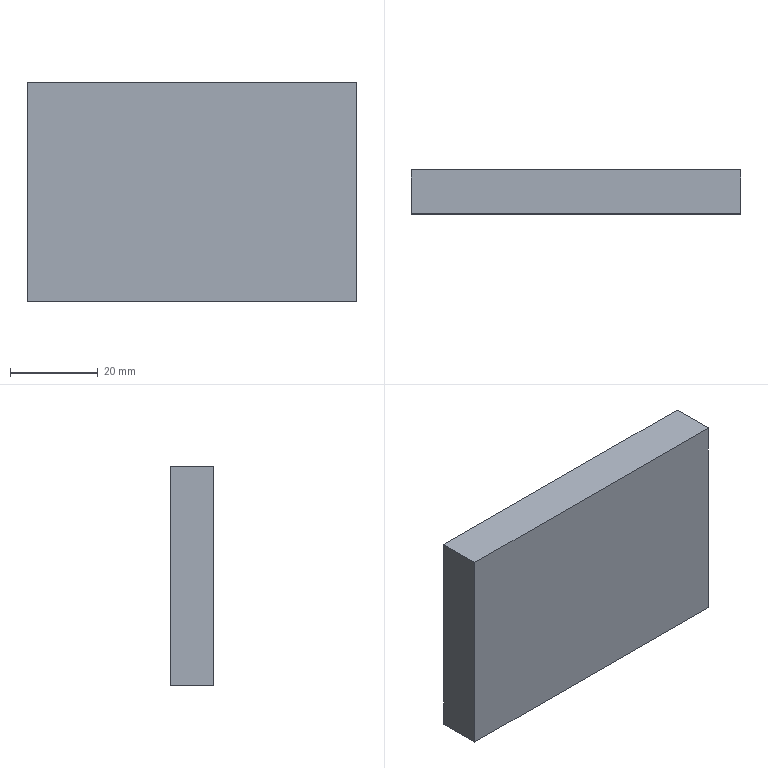Part | SolidWorks | features Extrusion 1 | 1 solid | 6 faces | box 75 x 10 x 50 mm | volume 37500 mm3 | plane 6
STEP:
#1=CARTESIAN_POINT('',(37.5,0.,25.));
#2=VERTEX_POINT('',#1);
#3=CARTESIAN_POINT('',(37.5,0.,-25.));
#4=VERTEX_POINT('',#3);
#5=CARTESIAN_POINT('',(37.5,0.,25.));
#6=DIRECTION('',(0.,0.,-1.));
#7=VECTOR('',#6,1000.);
#8=LINE('',#5,#7);
#9=EDGE_CURVE('',#2,#4,#8,.T.);
#10=ORIENTED_EDGE('',*,*,#9,.T.);
#11=CARTESIAN_POINT('',(37.5,10.,-25.));
#12=VERTEX_POINT('',#11);
#13=CARTESIAN_POINT('',(37.5,10.,-25.));
#14=DIRECTION('',(0.,-1.,0.));
#15=VECTOR('',#14,1000.);
#16=LINE('',#13,#15);
#17=EDGE_CURVE('',#12,#4,#16,.T.);
#18=ORIENTED_EDGE('',*,*,#17,.F.);
#19=CARTESIAN_POINT('',(37.5,10.,25.));
#20=VERTEX_POINT('',#19);
#21=CARTESIAN_POINT('',(37.5,10.,25.));
#22=DIRECTION('',(0.,0.,-1.));
#23=VECTOR('',#22,1000.);
#24=LINE('',#21,#23);
#25=EDGE_CURVE('',#20,#12,#24,.T.);
#26=ORIENTED_EDGE('',*,*,#25,.F.);
#27=CARTESIAN_POINT('',(37.5,10.,25.));
#28=DIRECTION('',(0.,-1.,0.));
#29=VECTOR('',#28,1000.);
#30=LINE('',#27,#29);
#31=EDGE_CURVE('',#20,#2,#30,.T.);
#32=ORIENTED_EDGE('',*,*,#31,.T.);
#33=EDGE_LOOP('',(#10,#18,#26,#32));
#34=FACE_OUTER_BOUND('',#33,.T.);
#35=CARTESIAN_POINT('',(37.5,10.,25.));
#36=DIRECTION('',(-1.,0.,0.));
#37=DIRECTION('',(0.,0.,1.));
#38=AXIS2_PLACEMENT_3D('',#35,#36,#37);
#39=PLANE('',#38);
#40=ADVANCED_FACE('',(#34),#39,.F.);
#41=CARTESIAN_POINT('',(-37.5,0.,-25.));
#42=VERTEX_POINT('',#41);
#43=CARTESIAN_POINT('',(-37.5,0.,-25.));
#44=DIRECTION('',(-1.,0.,0.));
#45=VECTOR('',#44,1000.);
#46=LINE('',#43,#45);
#47=EDGE_CURVE('',#4,#42,#46,.T.);
#48=ORIENTED_EDGE('',*,*,#47,.T.);
#49=CARTESIAN_POINT('',(-37.5,10.,-25.));
#50=VERTEX_POINT('',#49);
#51=CARTESIAN_POINT('',(-37.5,10.,-25.));
#52=DIRECTION('',(0.,-1.,0.));
#53=VECTOR('',#52,1000.);
#54=LINE('',#51,#53);
#55=EDGE_CURVE('',#50,#42,#54,.T.);
#56=ORIENTED_EDGE('',*,*,#55,.F.);
#57=CARTESIAN_POINT('',(-37.5,10.,-25.));
#58=DIRECTION('',(-1.,0.,0.));
#59=VECTOR('',#58,1000.);
#60=LINE('',#57,#59);
#61=EDGE_CURVE('',#12,#50,#60,.T.);
#62=ORIENTED_EDGE('',*,*,#61,.F.);
#63=ORIENTED_EDGE('',*,*,#17,.T.);
#64=EDGE_LOOP('',(#48,#56,#62,#63));
#65=FACE_OUTER_BOUND('',#64,.T.);
#66=CARTESIAN_POINT('',(-37.5,10.,-25.));
#67=DIRECTION('',(0.,0.,1.));
#68=DIRECTION('',(1.,0.,0.));
#69=AXIS2_PLACEMENT_3D('',#66,#67,#68);
#70=PLANE('',#69);
#71=ADVANCED_FACE('',(#65),#70,.F.);
#72=CARTESIAN_POINT('',(-37.5,0.,25.));
#73=VERTEX_POINT('',#72);
#74=CARTESIAN_POINT('',(-37.5,0.,25.));
#75=DIRECTION('',(0.,0.,1.));
#76=VECTOR('',#75,1000.);
#77=LINE('',#74,#76);
#78=EDGE_CURVE('',#42,#73,#77,.T.);
#79=ORIENTED_EDGE('',*,*,#78,.T.);
#80=CARTESIAN_POINT('',(-37.5,10.,25.));
#81=VERTEX_POINT('',#80);
#82=CARTESIAN_POINT('',(-37.5,10.,25.));
#83=DIRECTION('',(0.,-1.,0.));
#84=VECTOR('',#83,1000.);
#85=LINE('',#82,#84);
#86=EDGE_CURVE('',#81,#73,#85,.T.);
#87=ORIENTED_EDGE('',*,*,#86,.F.);
#88=CARTESIAN_POINT('',(-37.5,10.,25.));
#89=DIRECTION('',(0.,0.,1.));
#90=VECTOR('',#89,1000.);
#91=LINE('',#88,#90);
#92=EDGE_CURVE('',#50,#81,#91,.T.);
#93=ORIENTED_EDGE('',*,*,#92,.F.);
#94=ORIENTED_EDGE('',*,*,#55,.T.);
#95=EDGE_LOOP('',(#79,#87,#93,#94));
#96=FACE_OUTER_BOUND('',#95,.T.);
#97=CARTESIAN_POINT('',(-37.5,10.,25.));
#98=DIRECTION('',(1.,0.,0.));
#99=DIRECTION('',(0.,0.,-1.));
#100=AXIS2_PLACEMENT_3D('',#97,#98,#99);
#101=PLANE('',#100);
#102=ADVANCED_FACE('',(#96),#101,.F.);
#103=CARTESIAN_POINT('',(-37.5,0.,25.));
#104=DIRECTION('',(1.,0.,0.));
#105=VECTOR('',#104,1000.);
#106=LINE('',#103,#105);
#107=EDGE_CURVE('',#73,#2,#106,.T.);
#108=ORIENTED_EDGE('',*,*,#107,.T.);
#109=ORIENTED_EDGE('',*,*,#31,.F.);
#110=CARTESIAN_POINT('',(-37.5,10.,25.));
#111=DIRECTION('',(1.,0.,0.));
#112=VECTOR('',#111,1000.);
#113=LINE('',#110,#112);
#114=EDGE_CURVE('',#81,#20,#113,.T.);
#115=ORIENTED_EDGE('',*,*,#114,.F.);
#116=ORIENTED_EDGE('',*,*,#86,.T.);
#117=EDGE_LOOP('',(#108,#109,#115,#116));
#118=FACE_OUTER_BOUND('',#117,.T.);
#119=CARTESIAN_POINT('',(-37.5,10.,25.));
#120=DIRECTION('',(0.,0.,-1.));
#121=DIRECTION('',(-1.,0.,0.));
#122=AXIS2_PLACEMENT_3D('',#119,#120,#121);
#123=PLANE('',#122);
#124=ADVANCED_FACE('',(#118),#123,.F.);
#125=ORIENTED_EDGE('',*,*,#25,.T.);
#126=ORIENTED_EDGE('',*,*,#61,.T.);
#127=ORIENTED_EDGE('',*,*,#92,.T.);
#128=ORIENTED_EDGE('',*,*,#114,.T.);
#129=EDGE_LOOP('',(#125,#126,#127,#128));
#130=FACE_OUTER_BOUND('',#129,.T.);
#131=CARTESIAN_POINT('',(0.,10.,0.));
#132=DIRECTION('',(0.,-1.,0.));
#133=DIRECTION('',(0.,0.,-1.));
#134=AXIS2_PLACEMENT_3D('',#131,#132,#133);
#135=PLANE('',#134);
#136=ADVANCED_FACE('',(#130),#135,.F.);
#137=ORIENTED_EDGE('',*,*,#9,.F.);
#138=ORIENTED_EDGE('',*,*,#107,.F.);
#139=ORIENTED_EDGE('',*,*,#78,.F.);
#140=ORIENTED_EDGE('',*,*,#47,.F.);
#141=EDGE_LOOP('',(#137,#138,#139,#140));
#142=FACE_OUTER_BOUND('',#141,.T.);
#143=CARTESIAN_POINT('',(0.,0.,0.));
#144=DIRECTION('',(0.,-1.,0.));
#145=DIRECTION('',(0.,0.,-1.));
#146=AXIS2_PLACEMENT_3D('',#143,#144,#145);
#147=PLANE('',#146);
#148=ADVANCED_FACE('',(#142),#147,.T.);
#149=CLOSED_SHELL('',(#40,#71,#102,#124,#136,#148));
#150=MANIFOLD_SOLID_BREP('',#149);
#151=CARTESIAN_POINT('',(0.,0.,0.));
#152=DIRECTION('',(0.,0.,1.));
#153=DIRECTION('',(1.,0.,0.));
#154=AXIS2_PLACEMENT_3D('',#151,#152,#153);
#155=(LENGTH_UNIT()NAMED_UNIT(*)SI_UNIT(.MILLI.,.METRE.));
#156=UNCERTAINTY_MEASURE_WITH_UNIT(LENGTH_MEASURE(0.00001),#155,'','');
#157=(NAMED_UNIT(*)PLANE_ANGLE_UNIT()SI_UNIT($,.RADIAN.));
#158=(NAMED_UNIT(*)SI_UNIT($,.STERADIAN.)SOLID_ANGLE_UNIT());
#159=(GEOMETRIC_REPRESENTATION_CONTEXT(3)GLOBAL_UNCERTAINTY_ASSIGNED_CONTEXT((#156))GLOBAL_UNIT_ASSIGNED_CONTEXT((#155,#157,#158))REPRESENTATION_CONTEXT('',''));
#160=ADVANCED_BREP_SHAPE_REPRESENTATION('',(#150,#154),#159);